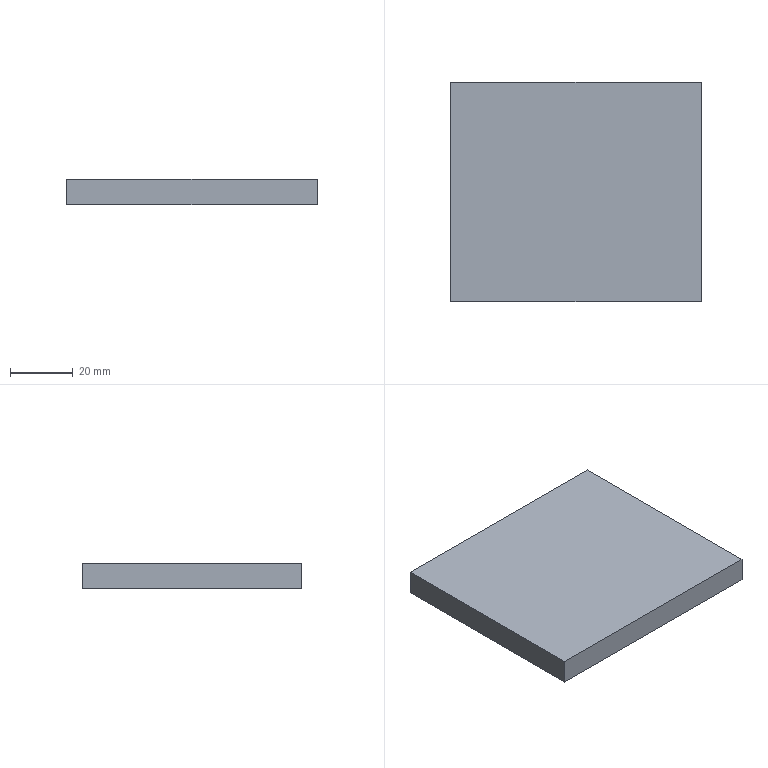Part | SolidWorks | features BaseBody 1 | 1 solid | 6 faces | box 80 x 70 x 8 mm | volume 44800 mm3 | plane 6
STEP:
#1=CARTESIAN_POINT('',(40.,-35.,-4.));
#2=VERTEX_POINT('',#1);
#3=CARTESIAN_POINT('',(40.,35.,-4.));
#4=VERTEX_POINT('',#3);
#5=CARTESIAN_POINT('',(40.,-35.,-4.));
#6=DIRECTION('',(0.,1.,0.));
#7=VECTOR('',#6,1000.);
#8=LINE('',#5,#7);
#9=EDGE_CURVE('',#2,#4,#8,.T.);
#10=ORIENTED_EDGE('',*,*,#9,.F.);
#11=CARTESIAN_POINT('',(-40.,-35.,-4.));
#12=VERTEX_POINT('',#11);
#13=CARTESIAN_POINT('',(-40.,-35.,-4.));
#14=DIRECTION('',(1.,0.,0.));
#15=VECTOR('',#14,1000.);
#16=LINE('',#13,#15);
#17=EDGE_CURVE('',#12,#2,#16,.T.);
#18=ORIENTED_EDGE('',*,*,#17,.F.);
#19=CARTESIAN_POINT('',(-40.,35.,-4.));
#20=VERTEX_POINT('',#19);
#21=CARTESIAN_POINT('',(-40.,-35.,-4.));
#22=DIRECTION('',(0.,-1.,0.));
#23=VECTOR('',#22,1000.);
#24=LINE('',#21,#23);
#25=EDGE_CURVE('',#20,#12,#24,.T.);
#26=ORIENTED_EDGE('',*,*,#25,.F.);
#27=CARTESIAN_POINT('',(-40.,35.,-4.));
#28=DIRECTION('',(-1.,0.,0.));
#29=VECTOR('',#28,1000.);
#30=LINE('',#27,#29);
#31=EDGE_CURVE('',#4,#20,#30,.T.);
#32=ORIENTED_EDGE('',*,*,#31,.F.);
#33=EDGE_LOOP('',(#10,#18,#26,#32));
#34=FACE_OUTER_BOUND('',#33,.T.);
#35=CARTESIAN_POINT('',(-40.,-35.,-4.));
#36=DIRECTION('',(0.,0.,1.));
#37=DIRECTION('',(1.,0.,0.));
#38=AXIS2_PLACEMENT_3D('',#35,#36,#37);
#39=PLANE('',#38);
#40=ADVANCED_FACE('',(#34),#39,.F.);
#41=CARTESIAN_POINT('',(-40.,35.,4.));
#42=VERTEX_POINT('',#41);
#43=CARTESIAN_POINT('',(40.,35.,4.));
#44=VERTEX_POINT('',#43);
#45=CARTESIAN_POINT('',(-40.,35.,4.));
#46=DIRECTION('',(1.,0.,0.));
#47=VECTOR('',#46,1000.);
#48=LINE('',#45,#47);
#49=EDGE_CURVE('',#42,#44,#48,.T.);
#50=ORIENTED_EDGE('',*,*,#49,.T.);
#51=CARTESIAN_POINT('',(40.,35.,-4.));
#52=DIRECTION('',(0.,0.,-1.));
#53=VECTOR('',#52,1000.);
#54=LINE('',#51,#53);
#55=EDGE_CURVE('',#44,#4,#54,.T.);
#56=ORIENTED_EDGE('',*,*,#55,.T.);
#57=ORIENTED_EDGE('',*,*,#31,.T.);
#58=CARTESIAN_POINT('',(-40.,35.,-4.));
#59=DIRECTION('',(0.,0.,1.));
#60=VECTOR('',#59,1000.);
#61=LINE('',#58,#60);
#62=EDGE_CURVE('',#20,#42,#61,.T.);
#63=ORIENTED_EDGE('',*,*,#62,.T.);
#64=EDGE_LOOP('',(#50,#56,#57,#63));
#65=FACE_OUTER_BOUND('',#64,.T.);
#66=CARTESIAN_POINT('',(-40.,35.,-4.));
#67=DIRECTION('',(0.,1.,0.));
#68=DIRECTION('',(0.,0.,1.));
#69=AXIS2_PLACEMENT_3D('',#66,#67,#68);
#70=PLANE('',#69);
#71=ADVANCED_FACE('',(#65),#70,.T.);
#72=ORIENTED_EDGE('',*,*,#55,.F.);
#73=CARTESIAN_POINT('',(40.,-35.,4.));
#74=VERTEX_POINT('',#73);
#75=CARTESIAN_POINT('',(40.,-35.,4.));
#76=DIRECTION('',(0.,-1.,0.));
#77=VECTOR('',#76,1000.);
#78=LINE('',#75,#77);
#79=EDGE_CURVE('',#44,#74,#78,.T.);
#80=ORIENTED_EDGE('',*,*,#79,.T.);
#81=CARTESIAN_POINT('',(40.,-35.,-4.));
#82=DIRECTION('',(0.,0.,-1.));
#83=VECTOR('',#82,1000.);
#84=LINE('',#81,#83);
#85=EDGE_CURVE('',#74,#2,#84,.T.);
#86=ORIENTED_EDGE('',*,*,#85,.T.);
#87=ORIENTED_EDGE('',*,*,#9,.T.);
#88=EDGE_LOOP('',(#72,#80,#86,#87));
#89=FACE_OUTER_BOUND('',#88,.T.);
#90=CARTESIAN_POINT('',(40.,-35.,-4.));
#91=DIRECTION('',(1.,0.,0.));
#92=DIRECTION('',(0.,0.,-1.));
#93=AXIS2_PLACEMENT_3D('',#90,#91,#92);
#94=PLANE('',#93);
#95=ADVANCED_FACE('',(#89),#94,.T.);
#96=CARTESIAN_POINT('',(-40.,-35.,4.));
#97=VERTEX_POINT('',#96);
#98=CARTESIAN_POINT('',(-40.,-35.,4.));
#99=DIRECTION('',(1.,0.,0.));
#100=VECTOR('',#99,1000.);
#101=LINE('',#98,#100);
#102=EDGE_CURVE('',#97,#74,#101,.T.);
#103=ORIENTED_EDGE('',*,*,#102,.F.);
#104=CARTESIAN_POINT('',(-40.,-35.,-4.));
#105=DIRECTION('',(0.,0.,1.));
#106=VECTOR('',#105,1000.);
#107=LINE('',#104,#106);
#108=EDGE_CURVE('',#12,#97,#107,.T.);
#109=ORIENTED_EDGE('',*,*,#108,.F.);
#110=ORIENTED_EDGE('',*,*,#17,.T.);
#111=ORIENTED_EDGE('',*,*,#85,.F.);
#112=EDGE_LOOP('',(#103,#109,#110,#111));
#113=FACE_OUTER_BOUND('',#112,.T.);
#114=CARTESIAN_POINT('',(-40.,-35.,-4.));
#115=DIRECTION('',(0.,1.,0.));
#116=DIRECTION('',(0.,0.,1.));
#117=AXIS2_PLACEMENT_3D('',#114,#115,#116);
#118=PLANE('',#117);
#119=ADVANCED_FACE('',(#113),#118,.F.);
#120=ORIENTED_EDGE('',*,*,#62,.F.);
#121=ORIENTED_EDGE('',*,*,#25,.T.);
#122=ORIENTED_EDGE('',*,*,#108,.T.);
#123=CARTESIAN_POINT('',(-40.,-35.,4.));
#124=DIRECTION('',(0.,-1.,0.));
#125=VECTOR('',#124,1000.);
#126=LINE('',#123,#125);
#127=EDGE_CURVE('',#42,#97,#126,.T.);
#128=ORIENTED_EDGE('',*,*,#127,.F.);
#129=EDGE_LOOP('',(#120,#121,#122,#128));
#130=FACE_OUTER_BOUND('',#129,.T.);
#131=CARTESIAN_POINT('',(-40.,-35.,-4.));
#132=DIRECTION('',(1.,0.,0.));
#133=DIRECTION('',(0.,0.,-1.));
#134=AXIS2_PLACEMENT_3D('',#131,#132,#133);
#135=PLANE('',#134);
#136=ADVANCED_FACE('',(#130),#135,.F.);
#137=ORIENTED_EDGE('',*,*,#79,.F.);
#138=ORIENTED_EDGE('',*,*,#49,.F.);
#139=ORIENTED_EDGE('',*,*,#127,.T.);
#140=ORIENTED_EDGE('',*,*,#102,.T.);
#141=EDGE_LOOP('',(#137,#138,#139,#140));
#142=FACE_OUTER_BOUND('',#141,.T.);
#143=CARTESIAN_POINT('',(-40.,-35.,4.));
#144=DIRECTION('',(0.,0.,1.));
#145=DIRECTION('',(1.,0.,0.));
#146=AXIS2_PLACEMENT_3D('',#143,#144,#145);
#147=PLANE('',#146);
#148=ADVANCED_FACE('',(#142),#147,.T.);
#149=CLOSED_SHELL('',(#40,#71,#95,#119,#136,#148));
#150=MANIFOLD_SOLID_BREP('',#149);
#151=CARTESIAN_POINT('',(0.,0.,0.));
#152=DIRECTION('',(0.,0.,1.));
#153=DIRECTION('',(1.,0.,0.));
#154=AXIS2_PLACEMENT_3D('',#151,#152,#153);
#155=(LENGTH_UNIT()NAMED_UNIT(*)SI_UNIT(.MILLI.,.METRE.));
#156=UNCERTAINTY_MEASURE_WITH_UNIT(LENGTH_MEASURE(0.00001),#155,'','');
#157=(NAMED_UNIT(*)PLANE_ANGLE_UNIT()SI_UNIT($,.RADIAN.));
#158=(NAMED_UNIT(*)SI_UNIT($,.STERADIAN.)SOLID_ANGLE_UNIT());
#159=(GEOMETRIC_REPRESENTATION_CONTEXT(3)GLOBAL_UNCERTAINTY_ASSIGNED_CONTEXT((#156))GLOBAL_UNIT_ASSIGNED_CONTEXT((#155,#157,#158))REPRESENTATION_CONTEXT('',''));
#160=ADVANCED_BREP_SHAPE_REPRESENTATION('',(#150,#154),#159);